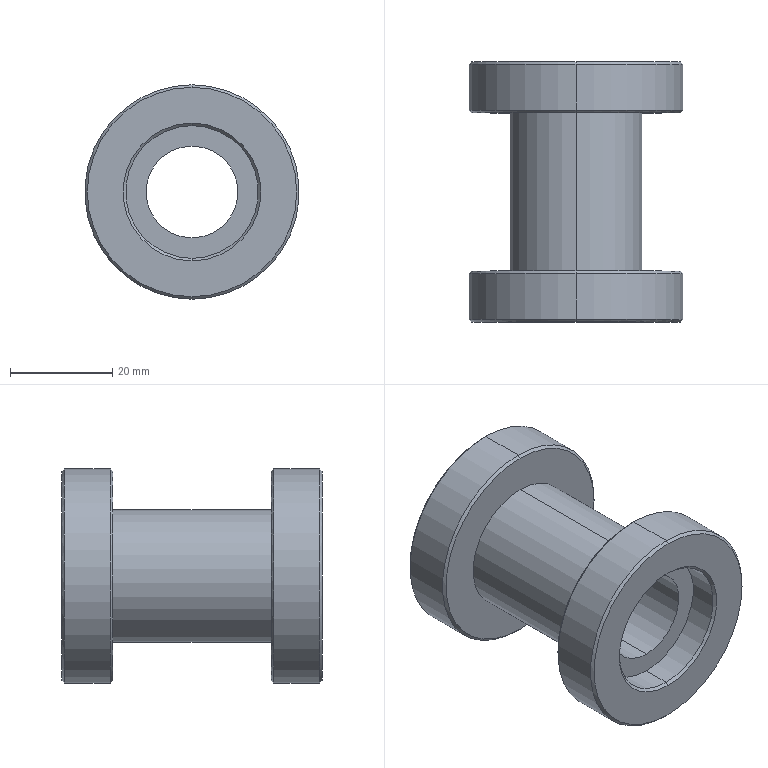Part | STEP file | adjusting belt tension wheel 2_SUS304 | 1 solid | 30 faces | box 42 x 51 x 42 mm | volume 27786 mm3 | cylinder 12 | cone 12 | plane 6 | commonest cylinder face diameters 26 x6 42 x4 18 x2